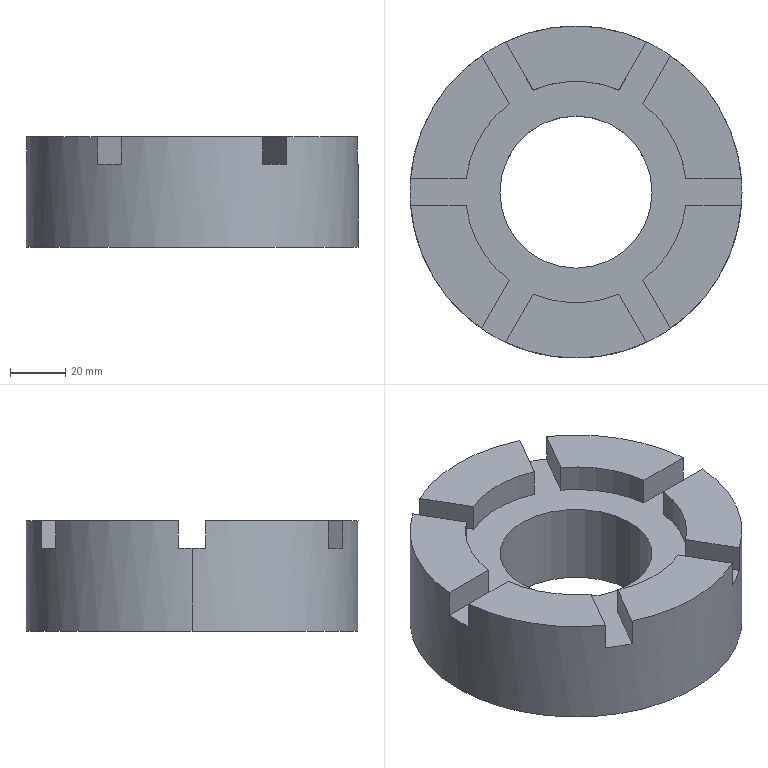Part | SolidWorks | features ICE 3, CirPattern 1, Extrusion 1 | 1 solid | 30 faces | box 120 x 120 x 40 mm | volume 318828 mm3 | plane 20 | cylinder 10 | commonest cylinder face diameters 80 x6 55 x2 120 x2
STEP:
#1=CARTESIAN_POINT('',(27.5,0.,0.));
#2=VERTEX_POINT('',#1);
#3=CARTESIAN_POINT('',(-27.5,0.,0.));
#4=VERTEX_POINT('',#3);
#5=CARTESIAN_POINT('',(0.,0.,0.));
#6=DIRECTION('',(0.,0.,-1.));
#7=DIRECTION('',(1.,0.,0.));
#8=AXIS2_PLACEMENT_3D('',#5,#6,#7);
#9=CIRCLE('',#8,27.5);
#10=EDGE_CURVE('',#2,#4,#9,.T.);
#11=ORIENTED_EDGE('',*,*,#10,.T.);
#12=CARTESIAN_POINT('',(-27.5,0.,30.));
#13=VERTEX_POINT('',#12);
#14=CARTESIAN_POINT('',(-27.5,0.,-0.001));
#15=DIRECTION('',(0.,0.,1.));
#16=VECTOR('',#15,1000.);
#17=LINE('',#14,#16);
#18=EDGE_CURVE('',#4,#13,#17,.T.);
#19=ORIENTED_EDGE('',*,*,#18,.T.);
#20=CARTESIAN_POINT('',(27.5,0.,30.));
#21=VERTEX_POINT('',#20);
#22=CARTESIAN_POINT('',(0.,0.,30.));
#23=DIRECTION('',(0.,0.,1.));
#24=DIRECTION('',(1.,0.,0.));
#25=AXIS2_PLACEMENT_3D('',#22,#23,#24);
#26=CIRCLE('',#25,27.5);
#27=EDGE_CURVE('',#13,#21,#26,.T.);
#28=ORIENTED_EDGE('',*,*,#27,.T.);
#29=CARTESIAN_POINT('',(27.5,0.,-0.001));
#30=DIRECTION('',(0.,0.,1.));
#31=VECTOR('',#30,1000.);
#32=LINE('',#29,#31);
#33=EDGE_CURVE('',#2,#21,#32,.T.);
#34=ORIENTED_EDGE('',*,*,#33,.F.);
#35=EDGE_LOOP('',(#11,#19,#28,#34));
#36=FACE_OUTER_BOUND('',#35,.T.);
#37=CARTESIAN_POINT('',(0.,0.,-0.001));
#38=DIRECTION('',(0.,0.,1.));
#39=DIRECTION('',(1.,0.,0.));
#40=AXIS2_PLACEMENT_3D('',#37,#38,#39);
#41=CYLINDRICAL_SURFACE('',#40,27.5);
#42=ADVANCED_FACE('',(#36),#41,.F.);
#43=CARTESIAN_POINT('',(60.,0.,30.));
#44=VERTEX_POINT('',#43);
#45=CARTESIAN_POINT('',(59.791,5.,30.));
#46=VERTEX_POINT('',#45);
#47=CARTESIAN_POINT('',(0.,0.,30.));
#48=DIRECTION('',(0.,0.,1.));
#49=DIRECTION('',(-1.,0.,0.));
#50=AXIS2_PLACEMENT_3D('',#47,#48,#49);
#51=CIRCLE('',#50,60.);
#52=EDGE_CURVE('',#44,#46,#51,.T.);
#53=ORIENTED_EDGE('',*,*,#52,.F.);
#54=CARTESIAN_POINT('',(60.,0.,0.));
#55=VERTEX_POINT('',#54);
#56=CARTESIAN_POINT('',(60.,0.,40.));
#57=DIRECTION('',(0.,0.,-1.));
#58=VECTOR('',#57,1000.);
#59=LINE('',#56,#58);
#60=EDGE_CURVE('',#44,#55,#59,.T.);
#61=ORIENTED_EDGE('',*,*,#60,.T.);
#62=CARTESIAN_POINT('',(-60.,0.,0.));
#63=VERTEX_POINT('',#62);
#64=CARTESIAN_POINT('',(0.,0.,0.));
#65=DIRECTION('',(0.,0.,1.));
#66=DIRECTION('',(1.,0.,0.));
#67=AXIS2_PLACEMENT_3D('',#64,#65,#66);
#68=CIRCLE('',#67,60.);
#69=EDGE_CURVE('',#55,#63,#68,.T.);
#70=ORIENTED_EDGE('',*,*,#69,.T.);
#71=CARTESIAN_POINT('',(-60.,0.,30.));
#72=VERTEX_POINT('',#71);
#73=CARTESIAN_POINT('',(-60.,0.,40.));
#74=DIRECTION('',(0.,0.,-1.));
#75=VECTOR('',#74,1000.);
#76=LINE('',#73,#75);
#77=EDGE_CURVE('',#72,#63,#76,.T.);
#78=ORIENTED_EDGE('',*,*,#77,.F.);
#79=CARTESIAN_POINT('',(-59.791,5.,30.));
#80=VERTEX_POINT('',#79);
#81=CARTESIAN_POINT('',(0.,0.,30.));
#82=DIRECTION('',(0.,0.,1.));
#83=DIRECTION('',(-1.,0.,0.));
#84=AXIS2_PLACEMENT_3D('',#81,#82,#83);
#85=CIRCLE('',#84,60.);
#86=EDGE_CURVE('',#80,#72,#85,.T.);
#87=ORIENTED_EDGE('',*,*,#86,.F.);
#88=CARTESIAN_POINT('',(-59.791,5.,40.));
#89=VERTEX_POINT('',#88);
#90=CARTESIAN_POINT('',(-59.791,5.,40.));
#91=DIRECTION('',(0.,0.,1.));
#92=VECTOR('',#91,1000.);
#93=LINE('',#90,#92);
#94=EDGE_CURVE('',#80,#89,#93,.T.);
#95=ORIENTED_EDGE('',*,*,#94,.T.);
#96=CARTESIAN_POINT('',(-34.226,49.281,40.));
#97=VERTEX_POINT('',#96);
#98=CARTESIAN_POINT('',(0.,0.,40.));
#99=DIRECTION('',(0.,0.,1.));
#100=DIRECTION('',(1.,0.,0.));
#101=AXIS2_PLACEMENT_3D('',#98,#99,#100);
#102=CIRCLE('',#101,60.);
#103=EDGE_CURVE('',#97,#89,#102,.T.);
#104=ORIENTED_EDGE('',*,*,#103,.F.);
#105=CARTESIAN_POINT('',(-34.226,49.281,30.));
#106=VERTEX_POINT('',#105);
#107=CARTESIAN_POINT('',(-34.226,49.281,40.));
#108=DIRECTION('',(0.,0.,-1.));
#109=VECTOR('',#108,1000.);
#110=LINE('',#107,#109);
#111=EDGE_CURVE('',#97,#106,#110,.T.);
#112=ORIENTED_EDGE('',*,*,#111,.T.);
#113=CARTESIAN_POINT('',(-25.566,54.281,30.));
#114=VERTEX_POINT('',#113);
#115=CARTESIAN_POINT('',(0.,0.,30.));
#116=DIRECTION('',(0.,0.,1.));
#117=DIRECTION('',(-1.,0.,0.));
#118=AXIS2_PLACEMENT_3D('',#115,#116,#117);
#119=CIRCLE('',#118,60.);
#120=EDGE_CURVE('',#114,#106,#119,.T.);
#121=ORIENTED_EDGE('',*,*,#120,.F.);
#122=CARTESIAN_POINT('',(-25.566,54.281,40.));
#123=VERTEX_POINT('',#122);
#124=CARTESIAN_POINT('',(-25.566,54.281,40.));
#125=DIRECTION('',(0.,0.,1.));
#126=VECTOR('',#125,1000.);
#127=LINE('',#124,#126);
#128=EDGE_CURVE('',#114,#123,#127,.T.);
#129=ORIENTED_EDGE('',*,*,#128,.T.);
#130=CARTESIAN_POINT('',(25.566,54.281,40.));
#131=VERTEX_POINT('',#130);
#132=CARTESIAN_POINT('',(0.,0.,40.));
#133=DIRECTION('',(0.,0.,1.));
#134=DIRECTION('',(1.,0.,0.));
#135=AXIS2_PLACEMENT_3D('',#132,#133,#134);
#136=CIRCLE('',#135,60.);
#137=EDGE_CURVE('',#131,#123,#136,.T.);
#138=ORIENTED_EDGE('',*,*,#137,.F.);
#139=CARTESIAN_POINT('',(25.566,54.281,30.));
#140=VERTEX_POINT('',#139);
#141=CARTESIAN_POINT('',(25.566,54.281,40.));
#142=DIRECTION('',(0.,0.,-1.));
#143=VECTOR('',#142,1000.);
#144=LINE('',#141,#143);
#145=EDGE_CURVE('',#131,#140,#144,.T.);
#146=ORIENTED_EDGE('',*,*,#145,.T.);
#147=CARTESIAN_POINT('',(34.226,49.281,30.));
#148=VERTEX_POINT('',#147);
#149=CARTESIAN_POINT('',(0.,0.,30.));
#150=DIRECTION('',(0.,0.,1.));
#151=DIRECTION('',(-1.,0.,0.));
#152=AXIS2_PLACEMENT_3D('',#149,#150,#151);
#153=CIRCLE('',#152,60.);
#154=EDGE_CURVE('',#148,#140,#153,.T.);
#155=ORIENTED_EDGE('',*,*,#154,.F.);
#156=CARTESIAN_POINT('',(34.226,49.281,40.));
#157=VERTEX_POINT('',#156);
#158=CARTESIAN_POINT('',(34.226,49.281,40.));
#159=DIRECTION('',(0.,0.,1.));
#160=VECTOR('',#159,1000.);
#161=LINE('',#158,#160);
#162=EDGE_CURVE('',#148,#157,#161,.T.);
#163=ORIENTED_EDGE('',*,*,#162,.T.);
#164=CARTESIAN_POINT('',(59.791,5.,40.));
#165=VERTEX_POINT('',#164);
#166=CARTESIAN_POINT('',(0.,0.,40.));
#167=DIRECTION('',(0.,0.,1.));
#168=DIRECTION('',(1.,0.,0.));
#169=AXIS2_PLACEMENT_3D('',#166,#167,#168);
#170=CIRCLE('',#169,60.);
#171=EDGE_CURVE('',#165,#157,#170,.T.);
#172=ORIENTED_EDGE('',*,*,#171,.F.);
#173=CARTESIAN_POINT('',(59.791,5.,40.));
#174=DIRECTION('',(0.,0.,-1.));
#175=VECTOR('',#174,1000.);
#176=LINE('',#173,#175);
#177=EDGE_CURVE('',#165,#46,#176,.T.);
#178=ORIENTED_EDGE('',*,*,#177,.T.);
#179=EDGE_LOOP('',(#53,#61,#70,#78,#87,#95,#104,#112,#121,#129,#138,#146,#155,#163,#172,#178));
#180=FACE_OUTER_BOUND('',#179,.T.);
#181=CARTESIAN_POINT('',(0.,0.,40.));
#182=DIRECTION('',(0.,0.,-1.));
#183=DIRECTION('',(-1.,0.,0.));
#184=AXIS2_PLACEMENT_3D('',#181,#182,#183);
#185=CYLINDRICAL_SURFACE('',#184,60.);
#186=ADVANCED_FACE('',(#180),#185,.T.);
#187=ORIENTED_EDGE('',*,*,#60,.F.);
#188=CARTESIAN_POINT('',(59.791,-5.,30.));
#189=VERTEX_POINT('',#188);
#190=CARTESIAN_POINT('',(0.,0.,30.));
#191=DIRECTION('',(0.,0.,1.));
#192=DIRECTION('',(-1.,0.,0.));
#193=AXIS2_PLACEMENT_3D('',#190,#191,#192);
#194=CIRCLE('',#193,60.);
#195=EDGE_CURVE('',#189,#44,#194,.T.);
#196=ORIENTED_EDGE('',*,*,#195,.F.);
#197=CARTESIAN_POINT('',(59.791,-5.,40.));
#198=VERTEX_POINT('',#197);
#199=CARTESIAN_POINT('',(59.791,-5.,40.));
#200=DIRECTION('',(0.,0.,1.));
#201=VECTOR('',#200,1000.);
#202=LINE('',#199,#201);
#203=EDGE_CURVE('',#189,#198,#202,.T.);
#204=ORIENTED_EDGE('',*,*,#203,.T.);
#205=CARTESIAN_POINT('',(34.226,-49.281,40.));
#206=VERTEX_POINT('',#205);
#207=CARTESIAN_POINT('',(0.,0.,40.));
#208=DIRECTION('',(0.,0.,1.));
#209=DIRECTION('',(1.,0.,0.));
#210=AXIS2_PLACEMENT_3D('',#207,#208,#209);
#211=CIRCLE('',#210,60.);
#212=EDGE_CURVE('',#206,#198,#211,.T.);
#213=ORIENTED_EDGE('',*,*,#212,.F.);
#214=CARTESIAN_POINT('',(34.226,-49.281,30.));
#215=VERTEX_POINT('',#214);
#216=CARTESIAN_POINT('',(34.226,-49.281,40.));
#217=DIRECTION('',(0.,0.,-1.));
#218=VECTOR('',#217,1000.);
#219=LINE('',#216,#218);
#220=EDGE_CURVE('',#206,#215,#219,.T.);
#221=ORIENTED_EDGE('',*,*,#220,.T.);
#222=CARTESIAN_POINT('',(25.566,-54.281,30.));
#223=VERTEX_POINT('',#222);
#224=CARTESIAN_POINT('',(0.,0.,30.));
#225=DIRECTION('',(0.,0.,1.));
#226=DIRECTION('',(-1.,0.,0.));
#227=AXIS2_PLACEMENT_3D('',#224,#225,#226);
#228=CIRCLE('',#227,60.);
#229=EDGE_CURVE('',#223,#215,#228,.T.);
#230=ORIENTED_EDGE('',*,*,#229,.F.);
#231=CARTESIAN_POINT('',(25.566,-54.281,40.));
#232=VERTEX_POINT('',#231);
#233=CARTESIAN_POINT('',(25.566,-54.281,40.));
#234=DIRECTION('',(0.,0.,1.));
#235=VECTOR('',#234,1000.);
#236=LINE('',#233,#235);
#237=EDGE_CURVE('',#223,#232,#236,.T.);
#238=ORIENTED_EDGE('',*,*,#237,.T.);
#239=CARTESIAN_POINT('',(-25.566,-54.281,40.));
#240=VERTEX_POINT('',#239);
#241=CARTESIAN_POINT('',(0.,0.,40.));
#242=DIRECTION('',(0.,0.,1.));
#243=DIRECTION('',(1.,0.,0.));
#244=AXIS2_PLACEMENT_3D('',#241,#242,#243);
#245=CIRCLE('',#244,60.);
#246=EDGE_CURVE('',#240,#232,#245,.T.);
#247=ORIENTED_EDGE('',*,*,#246,.F.);
#248=CARTESIAN_POINT('',(-25.566,-54.281,30.));
#249=VERTEX_POINT('',#248);
#250=CARTESIAN_POINT('',(-25.566,-54.281,40.));
#251=DIRECTION('',(0.,0.,-1.));
#252=VECTOR('',#251,1000.);
#253=LINE('',#250,#252);
#254=EDGE_CURVE('',#240,#249,#253,.T.);
#255=ORIENTED_EDGE('',*,*,#254,.T.);
#256=CARTESIAN_POINT('',(-34.226,-49.281,30.));
#257=VERTEX_POINT('',#256);
#258=CARTESIAN_POINT('',(0.,0.,30.));
#259=DIRECTION('',(0.,0.,1.));
#260=DIRECTION('',(-1.,0.,0.));
#261=AXIS2_PLACEMENT_3D('',#258,#259,#260);
#262=CIRCLE('',#261,60.);
#263=EDGE_CURVE('',#257,#249,#262,.T.);
#264=ORIENTED_EDGE('',*,*,#263,.F.);
#265=CARTESIAN_POINT('',(-34.226,-49.281,40.));
#266=VERTEX_POINT('',#265);
#267=CARTESIAN_POINT('',(-34.226,-49.281,40.));
#268=DIRECTION('',(0.,0.,1.));
#269=VECTOR('',#268,1000.);
#270=LINE('',#267,#269);
#271=EDGE_CURVE('',#257,#266,#270,.T.);
#272=ORIENTED_EDGE('',*,*,#271,.T.);
#273=CARTESIAN_POINT('',(-59.791,-5.,40.));
#274=VERTEX_POINT('',#273);
#275=CARTESIAN_POINT('',(0.,0.,40.));
#276=DIRECTION('',(0.,0.,1.));
#277=DIRECTION('',(1.,0.,0.));
#278=AXIS2_PLACEMENT_3D('',#275,#276,#277);
#279=CIRCLE('',#278,60.);
#280=EDGE_CURVE('',#274,#266,#279,.T.);
#281=ORIENTED_EDGE('',*,*,#280,.F.);
#282=CARTESIAN_POINT('',(-59.791,-5.,30.));
#283=VERTEX_POINT('',#282);
#284=CARTESIAN_POINT('',(-59.791,-5.,40.));
#285=DIRECTION('',(0.,0.,-1.));
#286=VECTOR('',#285,1000.);
#287=LINE('',#284,#286);
#288=EDGE_CURVE('',#274,#283,#287,.T.);
#289=ORIENTED_EDGE('',*,*,#288,.T.);
#290=CARTESIAN_POINT('',(0.,0.,30.));
#291=DIRECTION('',(0.,0.,1.));
#292=DIRECTION('',(-1.,0.,0.));
#293=AXIS2_PLACEMENT_3D('',#290,#291,#292);
#294=CIRCLE('',#293,60.);
#295=EDGE_CURVE('',#72,#283,#294,.T.);
#296=ORIENTED_EDGE('',*,*,#295,.F.);
#297=ORIENTED_EDGE('',*,*,#77,.T.);
#298=CARTESIAN_POINT('',(0.,0.,0.));
#299=DIRECTION('',(0.,0.,1.));
#300=DIRECTION('',(1.,0.,0.));
#301=AXIS2_PLACEMENT_3D('',#298,#299,#300);
#302=CIRCLE('',#301,60.);
#303=EDGE_CURVE('',#63,#55,#302,.T.);
#304=ORIENTED_EDGE('',*,*,#303,.T.);
#305=EDGE_LOOP('',(#187,#196,#204,#213,#221,#230,#238,#247,#255,#264,#272,#281,#289,#296,#297,#304));
#306=FACE_OUTER_BOUND('',#305,.T.);
#307=CARTESIAN_POINT('',(0.,0.,40.));
#308=DIRECTION('',(0.,0.,-1.));
#309=DIRECTION('',(-1.,0.,0.));
#310=AXIS2_PLACEMENT_3D('',#307,#308,#309);
#311=CYLINDRICAL_SURFACE('',#310,60.);
#312=ADVANCED_FACE('',(#306),#311,.T.);
#313=ORIENTED_EDGE('',*,*,#246,.T.);
#314=CARTESIAN_POINT('',(15.513,-36.869,40.));
#315=VERTEX_POINT('',#314);
#316=CARTESIAN_POINT('',(33.17,-67.452,40.));
#317=DIRECTION('',(0.5,-0.866,0.));
#318=VECTOR('',#317,1000.);
#319=LINE('',#316,#318);
#320=EDGE_CURVE('',#315,#232,#319,.T.);
#321=ORIENTED_EDGE('',*,*,#320,.F.);
#322=CARTESIAN_POINT('',(-15.513,-36.869,40.));
#323=VERTEX_POINT('',#322);
#324=CARTESIAN_POINT('',(0.,0.,40.));
#325=DIRECTION('',(0.,0.,1.));
#326=DIRECTION('',(1.,0.,0.));
#327=AXIS2_PLACEMENT_3D('',#324,#325,#326);
#328=CIRCLE('',#327,40.);
#329=EDGE_CURVE('',#323,#315,#328,.T.);
#330=ORIENTED_EDGE('',*,*,#329,.F.);
#331=CARTESIAN_POINT('',(41.83,62.452,40.));
#332=DIRECTION('',(0.5,0.866,0.));
#333=VECTOR('',#332,1000.);
#334=LINE('',#331,#333);
#335=EDGE_CURVE('',#240,#323,#334,.T.);
#336=ORIENTED_EDGE('',*,*,#335,.F.);
#337=EDGE_LOOP('',(#313,#321,#330,#336));
#338=FACE_OUTER_BOUND('',#337,.T.);
#339=CARTESIAN_POINT('',(0.,0.,40.));
#340=DIRECTION('',(0.,0.,1.));
#341=DIRECTION('',(1.,0.,0.));
#342=AXIS2_PLACEMENT_3D('',#339,#340,#341);
#343=PLANE('',#342);
#344=ADVANCED_FACE('',(#338),#343,.T.);
#345=CARTESIAN_POINT('',(24.173,-31.869,40.));
#346=VERTEX_POINT('',#345);
#347=CARTESIAN_POINT('',(39.686,-5.,40.));
#348=VERTEX_POINT('',#347);
#349=CARTESIAN_POINT('',(0.,0.,40.));
#350=DIRECTION('',(0.,0.,1.));
#351=DIRECTION('',(1.,0.,0.));
#352=AXIS2_PLACEMENT_3D('',#349,#350,#351);
#353=CIRCLE('',#352,40.);
#354=EDGE_CURVE('',#346,#348,#353,.T.);
#355=ORIENTED_EDGE('',*,*,#354,.F.);
#356=CARTESIAN_POINT('',(41.83,-62.452,40.));
#357=DIRECTION('',(-0.5,0.866,0.));
#358=VECTOR('',#357,1000.);
#359=LINE('',#356,#358);
#360=EDGE_CURVE('',#206,#346,#359,.T.);
#361=ORIENTED_EDGE('',*,*,#360,.F.);
#362=ORIENTED_EDGE('',*,*,#212,.T.);
#363=CARTESIAN_POINT('',(-75.,-5.,40.));
#364=DIRECTION('',(1.,0.,0.));
#365=VECTOR('',#364,1000.);
#366=LINE('',#363,#365);
#367=EDGE_CURVE('',#348,#198,#366,.T.);
#368=ORIENTED_EDGE('',*,*,#367,.F.);
#369=EDGE_LOOP('',(#355,#361,#362,#368));
#370=FACE_OUTER_BOUND('',#369,.T.);
#371=CARTESIAN_POINT('',(0.,0.,40.));
#372=DIRECTION('',(0.,0.,1.));
#373=DIRECTION('',(1.,0.,0.));
#374=AXIS2_PLACEMENT_3D('',#371,#372,#373);
#375=PLANE('',#374);
#376=ADVANCED_FACE('',(#370),#375,.T.);
#377=ORIENTED_EDGE('',*,*,#280,.T.);
#378=CARTESIAN_POINT('',(-24.173,-31.869,40.));
#379=VERTEX_POINT('',#378);
#380=CARTESIAN_POINT('',(33.17,67.452,40.));
#381=DIRECTION('',(-0.5,-0.866,0.));
#382=VECTOR('',#381,1000.);
#383=LINE('',#380,#382);
#384=EDGE_CURVE('',#379,#266,#383,.T.);
#385=ORIENTED_EDGE('',*,*,#384,.F.);
#386=CARTESIAN_POINT('',(-39.686,-5.,40.));
#387=VERTEX_POINT('',#386);
#388=CARTESIAN_POINT('',(0.,0.,40.));
#389=DIRECTION('',(0.,0.,1.));
#390=DIRECTION('',(1.,0.,0.));
#391=AXIS2_PLACEMENT_3D('',#388,#389,#390);
#392=CIRCLE('',#391,40.);
#393=EDGE_CURVE('',#387,#379,#392,.T.);
#394=ORIENTED_EDGE('',*,*,#393,.F.);
#395=CARTESIAN_POINT('',(-75.,-5.,40.));
#396=DIRECTION('',(1.,0.,0.));
#397=VECTOR('',#396,1000.);
#398=LINE('',#395,#397);
#399=EDGE_CURVE('',#274,#387,#398,.T.);
#400=ORIENTED_EDGE('',*,*,#399,.F.);
#401=EDGE_LOOP('',(#377,#385,#394,#400));
#402=FACE_OUTER_BOUND('',#401,.T.);
#403=CARTESIAN_POINT('',(0.,0.,40.));
#404=DIRECTION('',(0.,0.,1.));
#405=DIRECTION('',(1.,0.,0.));
#406=AXIS2_PLACEMENT_3D('',#403,#404,#405);
#407=PLANE('',#406);
#408=ADVANCED_FACE('',(#402),#407,.T.);
#409=ORIENTED_EDGE('',*,*,#137,.T.);
#410=CARTESIAN_POINT('',(-15.513,36.869,40.));
#411=VERTEX_POINT('',#410);
#412=CARTESIAN_POINT('',(41.83,-62.452,40.));
#413=DIRECTION('',(-0.5,0.866,0.));
#414=VECTOR('',#413,1000.);
#415=LINE('',#412,#414);
#416=EDGE_CURVE('',#411,#123,#415,.T.);
#417=ORIENTED_EDGE('',*,*,#416,.F.);
#418=CARTESIAN_POINT('',(15.513,36.869,40.));
#419=VERTEX_POINT('',#418);
#420=CARTESIAN_POINT('',(0.,0.,40.));
#421=DIRECTION('',(0.,0.,1.));
#422=DIRECTION('',(1.,0.,0.));
#423=AXIS2_PLACEMENT_3D('',#420,#421,#422);
#424=CIRCLE('',#423,40.);
#425=EDGE_CURVE('',#419,#411,#424,.T.);
#426=ORIENTED_EDGE('',*,*,#425,.F.);
#427=CARTESIAN_POINT('',(33.17,67.452,40.));
#428=DIRECTION('',(-0.5,-0.866,0.));
#429=VECTOR('',#428,1000.);
#430=LINE('',#427,#429);
#431=EDGE_CURVE('',#131,#419,#430,.T.);
#432=ORIENTED_EDGE('',*,*,#431,.F.);
#433=EDGE_LOOP('',(#409,#417,#426,#432));
#434=FACE_OUTER_BOUND('',#433,.T.);
#435=CARTESIAN_POINT('',(0.,0.,40.));
#436=DIRECTION('',(0.,0.,1.));
#437=DIRECTION('',(1.,0.,0.));
#438=AXIS2_PLACEMENT_3D('',#435,#436,#437);
#439=PLANE('',#438);
#440=ADVANCED_FACE('',(#434),#439,.T.);
#441=CARTESIAN_POINT('',(-24.173,31.869,40.));
#442=VERTEX_POINT('',#441);
#443=CARTESIAN_POINT('',(-39.686,5.,40.));
#444=VERTEX_POINT('',#443);
#445=CARTESIAN_POINT('',(0.,0.,40.));
#446=DIRECTION('',(0.,0.,1.));
#447=DIRECTION('',(1.,0.,0.));
#448=AXIS2_PLACEMENT_3D('',#445,#446,#447);
#449=CIRCLE('',#448,40.);
#450=EDGE_CURVE('',#442,#444,#449,.T.);
#451=ORIENTED_EDGE('',*,*,#450,.F.);
#452=CARTESIAN_POINT('',(33.17,-67.452,40.));
#453=DIRECTION('',(0.5,-0.866,0.));
#454=VECTOR('',#453,1000.);
#455=LINE('',#452,#454);
#456=EDGE_CURVE('',#97,#442,#455,.T.);
#457=ORIENTED_EDGE('',*,*,#456,.F.);
#458=ORIENTED_EDGE('',*,*,#103,.T.);
#459=CARTESIAN_POINT('',(-75.,5.,40.));
#460=DIRECTION('',(-1.,0.,0.));
#461=VECTOR('',#460,1000.);
#462=LINE('',#459,#461);
#463=EDGE_CURVE('',#444,#89,#462,.T.);
#464=ORIENTED_EDGE('',*,*,#463,.F.);
#465=EDGE_LOOP('',(#451,#457,#458,#464));
#466=FACE_OUTER_BOUND('',#465,.T.);
#467=CARTESIAN_POINT('',(0.,0.,40.));
#468=DIRECTION('',(0.,0.,1.));
#469=DIRECTION('',(1.,0.,0.));
#470=AXIS2_PLACEMENT_3D('',#467,#468,#469);
#471=PLANE('',#470);
#472=ADVANCED_FACE('',(#466),#471,.T.);
#473=ORIENTED_EDGE('',*,*,#171,.T.);
#474=CARTESIAN_POINT('',(24.173,31.869,40.));
#475=VERTEX_POINT('',#474);
#476=CARTESIAN_POINT('',(41.83,62.452,40.));
#477=DIRECTION('',(0.5,0.866,0.));
#478=VECTOR('',#477,1000.);
#479=LINE('',#476,#478);
#480=EDGE_CURVE('',#475,#157,#479,.T.);
#481=ORIENTED_EDGE('',*,*,#480,.F.);
#482=CARTESIAN_POINT('',(39.686,5.,40.));
#483=VERTEX_POINT('',#482);
#484=CARTESIAN_POINT('',(0.,0.,40.));
#485=DIRECTION('',(0.,0.,1.));
#486=DIRECTION('',(1.,0.,0.));
#487=AXIS2_PLACEMENT_3D('',#484,#485,#486);
#488=CIRCLE('',#487,40.);
#489=EDGE_CURVE('',#483,#475,#488,.T.);
#490=ORIENTED_EDGE('',*,*,#489,.F.);
#491=CARTESIAN_POINT('',(-75.,5.,40.));
#492=DIRECTION('',(-1.,0.,0.));
#493=VECTOR('',#492,1000.);
#494=LINE('',#491,#493);
#495=EDGE_CURVE('',#165,#483,#494,.T.);
#496=ORIENTED_EDGE('',*,*,#495,.F.);
#497=EDGE_LOOP('',(#473,#481,#490,#496));
#498=FACE_OUTER_BOUND('',#497,.T.);
#499=CARTESIAN_POINT('',(0.,0.,40.));
#500=DIRECTION('',(0.,0.,1.));
#501=DIRECTION('',(1.,0.,0.));
#502=AXIS2_PLACEMENT_3D('',#499,#500,#501);
#503=PLANE('',#502);
#504=ADVANCED_FACE('',(#498),#503,.T.);
#505=CARTESIAN_POINT('',(15.513,-36.869,30.));
#506=VERTEX_POINT('',#505);
#507=CARTESIAN_POINT('',(15.513,-36.869,30.));
#508=DIRECTION('',(0.,0.,-1.));
#509=VECTOR('',#508,1000.);
#510=LINE('',#507,#509);
#511=EDGE_CURVE('',#315,#506,#510,.T.);
#512=ORIENTED_EDGE('',*,*,#511,.T.);
#513=CARTESIAN_POINT('',(-15.513,-36.869,30.));
#514=VERTEX_POINT('',#513);
#515=CARTESIAN_POINT('',(0.,0.,30.));
#516=DIRECTION('',(0.,0.,1.));
#517=DIRECTION('',(1.,0.,0.));
#518=AXIS2_PLACEMENT_3D('',#515,#516,#517);
#519=CIRCLE('',#518,40.);
#520=EDGE_CURVE('',#514,#506,#519,.T.);
#521=ORIENTED_EDGE('',*,*,#520,.F.);
#522=CARTESIAN_POINT('',(-15.513,-36.869,30.));
#523=DIRECTION('',(0.,0.,1.));
#524=VECTOR('',#523,1000.);
#525=LINE('',#522,#524);
#526=EDGE_CURVE('',#514,#323,#525,.T.);
#527=ORIENTED_EDGE('',*,*,#526,.T.);
#528=ORIENTED_EDGE('',*,*,#329,.T.);
#529=EDGE_LOOP('',(#512,#521,#527,#528));
#530=FACE_OUTER_BOUND('',#529,.T.);
#531=CARTESIAN_POINT('',(0.,0.,30.));
#532=DIRECTION('',(0.,0.,1.));
#533=DIRECTION('',(1.,0.,0.));
#534=AXIS2_PLACEMENT_3D('',#531,#532,#533);
#535=CYLINDRICAL_SURFACE('',#534,40.);
#536=ADVANCED_FACE('',(#530),#535,.F.);
#537=CARTESIAN_POINT('',(24.173,-31.869,30.));
#538=VERTEX_POINT('',#537);
#539=CARTESIAN_POINT('',(24.173,-31.869,30.));
#540=DIRECTION('',(0.,0.,1.));
#541=VECTOR('',#540,1000.);
#542=LINE('',#539,#541);
#543=EDGE_CURVE('',#538,#346,#542,.T.);
#544=ORIENTED_EDGE('',*,*,#543,.T.);
#545=ORIENTED_EDGE('',*,*,#354,.T.);
#546=CARTESIAN_POINT('',(39.686,-5.,30.));
#547=VERTEX_POINT('',#546);
#548=CARTESIAN_POINT('',(39.686,-5.,30.));
#549=DIRECTION('',(0.,0.,-1.));
#550=VECTOR('',#549,1000.);
#551=LINE('',#548,#550);
#552=EDGE_CURVE('',#348,#547,#551,.T.);
#553=ORIENTED_EDGE('',*,*,#552,.T.);
#554=CARTESIAN_POINT('',(0.,0.,30.));
#555=DIRECTION('',(0.,0.,1.));
#556=DIRECTION('',(1.,0.,0.));
#557=AXIS2_PLACEMENT_3D('',#554,#555,#556);
#558=CIRCLE('',#557,40.);
#559=EDGE_CURVE('',#538,#547,#558,.T.);
#560=ORIENTED_EDGE('',*,*,#559,.F.);
#561=EDGE_LOOP('',(#544,#545,#553,#560));
#562=FACE_OUTER_BOUND('',#561,.T.);
#563=CARTESIAN_POINT('',(0.,0.,30.));
#564=DIRECTION('',(0.,0.,1.));
#565=DIRECTION('',(1.,0.,0.));
#566=AXIS2_PLACEMENT_3D('',#563,#564,#565);
#567=CYLINDRICAL_SURFACE('',#566,40.);
#568=ADVANCED_FACE('',(#562),#567,.F.);
#569=CARTESIAN_POINT('',(-24.173,-31.869,30.));
#570=VERTEX_POINT('',#569);
#571=CARTESIAN_POINT('',(-24.173,-31.869,30.));
#572=DIRECTION('',(0.,0.,-1.));
#573=VECTOR('',#572,1000.);
#574=LINE('',#571,#573);
#575=EDGE_CURVE('',#379,#570,#574,.T.);
#576=ORIENTED_EDGE('',*,*,#575,.T.);
#577=CARTESIAN_POINT('',(-39.686,-5.,30.));
#578=VERTEX_POINT('',#577);
#579=CARTESIAN_POINT('',(0.,0.,30.));
#580=DIRECTION('',(0.,0.,1.));
#581=DIRECTION('',(1.,0.,0.));
#582=AXIS2_PLACEMENT_3D('',#579,#580,#581);
#583=CIRCLE('',#582,40.);
#584=EDGE_CURVE('',#578,#570,#583,.T.);
#585=ORIENTED_EDGE('',*,*,#584,.F.);
#586=CARTESIAN_POINT('',(-39.686,-5.,30.));
#587=DIRECTION('',(0.,0.,1.));
#588=VECTOR('',#587,1000.);
#589=LINE('',#586,#588);
#590=EDGE_CURVE('',#578,#387,#589,.T.);
#591=ORIENTED_EDGE('',*,*,#590,.T.);
#592=ORIENTED_EDGE('',*,*,#393,.T.);
#593=EDGE_LOOP('',(#576,#585,#591,#592));
#594=FACE_OUTER_BOUND('',#593,.T.);
#595=CARTESIAN_POINT('',(0.,0.,30.));
#596=DIRECTION('',(0.,0.,1.));
#597=DIRECTION('',(1.,0.,0.));
#598=AXIS2_PLACEMENT_3D('',#595,#596,#597);
#599=CYLINDRICAL_SURFACE('',#598,40.);
#600=ADVANCED_FACE('',(#594),#599,.F.);
#601=CARTESIAN_POINT('',(-15.513,36.869,30.));
#602=VERTEX_POINT('',#601);
#603=CARTESIAN_POINT('',(-15.513,36.869,30.));
#604=DIRECTION('',(0.,0.,-1.));
#605=VECTOR('',#604,1000.);
#606=LINE('',#603,#605);
#607=EDGE_CURVE('',#411,#602,#606,.T.);
#608=ORIENTED_EDGE('',*,*,#607,.T.);
#609=CARTESIAN_POINT('',(15.513,36.869,30.));
#610=VERTEX_POINT('',#609);
#611=CARTESIAN_POINT('',(0.,0.,30.));
#612=DIRECTION('',(0.,0.,1.));
#613=DIRECTION('',(1.,0.,0.));
#614=AXIS2_PLACEMENT_3D('',#611,#612,#613);
#615=CIRCLE('',#614,40.);
#616=EDGE_CURVE('',#610,#602,#615,.T.);
#617=ORIENTED_EDGE('',*,*,#616,.F.);
#618=CARTESIAN_POINT('',(15.513,36.869,30.));
#619=DIRECTION('',(0.,0.,1.));
#620=VECTOR('',#619,1000.);
#621=LINE('',#618,#620);
#622=EDGE_CURVE('',#610,#419,#621,.T.);
#623=ORIENTED_EDGE('',*,*,#622,.T.);
#624=ORIENTED_EDGE('',*,*,#425,.T.);
#625=EDGE_LOOP('',(#608,#617,#623,#624));
#626=FACE_OUTER_BOUND('',#625,.T.);
#627=CARTESIAN_POINT('',(0.,0.,30.));
#628=DIRECTION('',(0.,0.,1.));
#629=DIRECTION('',(1.,0.,0.));
#630=AXIS2_PLACEMENT_3D('',#627,#628,#629);
#631=CYLINDRICAL_SURFACE('',#630,40.);
#632=ADVANCED_FACE('',(#626),#631,.F.);
#633=CARTESIAN_POINT('',(-24.173,31.869,30.));
#634=VERTEX_POINT('',#633);
#635=CARTESIAN_POINT('',(-24.173,31.869,30.));
#636=DIRECTION('',(0.,0.,1.));
#637=VECTOR('',#636,1000.);
#638=LINE('',#635,#637);
#639=EDGE_CURVE('',#634,#442,#638,.T.);
#640=ORIENTED_EDGE('',*,*,#639,.T.);
#641=ORIENTED_EDGE('',*,*,#450,.T.);
#642=CARTESIAN_POINT('',(-39.686,5.,30.));
#643=VERTEX_POINT('',#642);
#644=CARTESIAN_POINT('',(-39.686,5.,30.));
#645=DIRECTION('',(0.,0.,-1.));
#646=VECTOR('',#645,1000.);
#647=LINE('',#644,#646);
#648=EDGE_CURVE('',#444,#643,#647,.T.);
#649=ORIENTED_EDGE('',*,*,#648,.T.);
#650=CARTESIAN_POINT('',(0.,0.,30.));
#651=DIRECTION('',(0.,0.,1.));
#652=DIRECTION('',(1.,0.,0.));
#653=AXIS2_PLACEMENT_3D('',#650,#651,#652);
#654=CIRCLE('',#653,40.);
#655=EDGE_CURVE('',#634,#643,#654,.T.);
#656=ORIENTED_EDGE('',*,*,#655,.F.);
#657=EDGE_LOOP('',(#640,#641,#649,#656));
#658=FACE_OUTER_BOUND('',#657,.T.);
#659=CARTESIAN_POINT('',(0.,0.,30.));
#660=DIRECTION('',(0.,0.,1.));
#661=DIRECTION('',(1.,0.,0.));
#662=AXIS2_PLACEMENT_3D('',#659,#660,#661);
#663=CYLINDRICAL_SURFACE('',#662,40.);
#664=ADVANCED_FACE('',(#658),#663,.F.);
#665=CARTESIAN_POINT('',(24.173,31.869,30.));
#666=VERTEX_POINT('',#665);
#667=CARTESIAN_POINT('',(24.173,31.869,30.));
#668=DIRECTION('',(0.,0.,-1.));
#669=VECTOR('',#668,1000.);
#670=LINE('',#667,#669);
#671=EDGE_CURVE('',#475,#666,#670,.T.);
#672=ORIENTED_EDGE('',*,*,#671,.T.);
#673=CARTESIAN_POINT('',(39.686,5.,30.));
#674=VERTEX_POINT('',#673);
#675=CARTESIAN_POINT('',(0.,0.,30.));
#676=DIRECTION('',(0.,0.,1.));
#677=DIRECTION('',(1.,0.,0.));
#678=AXIS2_PLACEMENT_3D('',#675,#676,#677);
#679=CIRCLE('',#678,40.);
#680=EDGE_CURVE('',#674,#666,#679,.T.);
#681=ORIENTED_EDGE('',*,*,#680,.F.);
#682=CARTESIAN_POINT('',(39.686,5.,30.));
#683=DIRECTION('',(0.,0.,1.));
#684=VECTOR('',#683,1000.);
#685=LINE('',#682,#684);
#686=EDGE_CURVE('',#674,#483,#685,.T.);
#687=ORIENTED_EDGE('',*,*,#686,.T.);
#688=ORIENTED_EDGE('',*,*,#489,.T.);
#689=EDGE_LOOP('',(#672,#681,#687,#688));
#690=FACE_OUTER_BOUND('',#689,.T.);
#691=CARTESIAN_POINT('',(0.,0.,30.));
#692=DIRECTION('',(0.,0.,1.));
#693=DIRECTION('',(1.,0.,0.));
#694=AXIS2_PLACEMENT_3D('',#691,#692,#693);
#695=CYLINDRICAL_SURFACE('',#694,40.);
#696=ADVANCED_FACE('',(#690),#695,.F.);
#697=ORIENTED_EDGE('',*,*,#10,.F.);
#698=CARTESIAN_POINT('',(0.,0.,0.));
#699=DIRECTION('',(0.,0.,-1.));
#700=DIRECTION('',(1.,0.,0.));
#701=AXIS2_PLACEMENT_3D('',#698,#699,#700);
#702=CIRCLE('',#701,27.5);
#703=EDGE_CURVE('',#4,#2,#702,.T.);
#704=ORIENTED_EDGE('',*,*,#703,.F.);
#705=EDGE_LOOP('',(#697,#704));
#706=FACE_BOUND('',#705,.T.);
#707=ORIENTED_EDGE('',*,*,#303,.F.);
#708=ORIENTED_EDGE('',*,*,#69,.F.);
#709=EDGE_LOOP('',(#707,#708));
#710=FACE_OUTER_BOUND('',#709,.T.);
#711=CARTESIAN_POINT('',(0.,0.,0.));
#712=DIRECTION('',(0.,0.,1.));
#713=DIRECTION('',(1.,0.,0.));
#714=AXIS2_PLACEMENT_3D('',#711,#712,#713);
#715=PLANE('',#714);
#716=ADVANCED_FACE('',(#706,#710),#715,.F.);
#717=CARTESIAN_POINT('',(0.,0.,30.));
#718=DIRECTION('',(0.,0.,1.));
#719=DIRECTION('',(1.,0.,0.));
#720=AXIS2_PLACEMENT_3D('',#717,#718,#719);
#721=CIRCLE('',#720,27.5);
#722=EDGE_CURVE('',#21,#13,#721,.T.);
#723=ORIENTED_EDGE('',*,*,#722,.F.);
#724=ORIENTED_EDGE('',*,*,#27,.F.);
#725=EDGE_LOOP('',(#723,#724));
#726=FACE_BOUND('',#725,.T.);
#727=ORIENTED_EDGE('',*,*,#680,.T.);
#728=CARTESIAN_POINT('',(41.83,62.452,30.));
#729=DIRECTION('',(0.5,0.866,0.));
#730=VECTOR('',#729,1000.);
#731=LINE('',#728,#730);
#732=EDGE_CURVE('',#666,#148,#731,.T.);
#733=ORIENTED_EDGE('',*,*,#732,.T.);
#734=ORIENTED_EDGE('',*,*,#154,.T.);
#735=CARTESIAN_POINT('',(33.17,67.452,30.));
#736=DIRECTION('',(-0.5,-0.866,0.));
#737=VECTOR('',#736,1000.);
#738=LINE('',#735,#737);
#739=EDGE_CURVE('',#140,#610,#738,.T.);
#740=ORIENTED_EDGE('',*,*,#739,.T.);
#741=ORIENTED_EDGE('',*,*,#616,.T.);
#742=CARTESIAN_POINT('',(41.83,-62.452,30.));
#743=DIRECTION('',(-0.5,0.866,0.));
#744=VECTOR('',#743,1000.);
#745=LINE('',#742,#744);
#746=EDGE_CURVE('',#602,#114,#745,.T.);
#747=ORIENTED_EDGE('',*,*,#746,.T.);
#748=ORIENTED_EDGE('',*,*,#120,.T.);
#749=CARTESIAN_POINT('',(33.17,-67.452,30.));
#750=DIRECTION('',(0.5,-0.866,0.));
#751=VECTOR('',#750,1000.);
#752=LINE('',#749,#751);
#753=EDGE_CURVE('',#106,#634,#752,.T.);
#754=ORIENTED_EDGE('',*,*,#753,.T.);
#755=ORIENTED_EDGE('',*,*,#655,.T.);
#756=CARTESIAN_POINT('',(-75.,5.,30.));
#757=DIRECTION('',(-1.,0.,0.));
#758=VECTOR('',#757,1000.);
#759=LINE('',#756,#758);
#760=EDGE_CURVE('',#643,#80,#759,.T.);
#761=ORIENTED_EDGE('',*,*,#760,.T.);
#762=ORIENTED_EDGE('',*,*,#86,.T.);
#763=ORIENTED_EDGE('',*,*,#295,.T.);
#764=CARTESIAN_POINT('',(-75.,-5.,30.));
#765=DIRECTION('',(1.,0.,0.));
#766=VECTOR('',#765,1000.);
#767=LINE('',#764,#766);
#768=EDGE_CURVE('',#283,#578,#767,.T.);
#769=ORIENTED_EDGE('',*,*,#768,.T.);
#770=ORIENTED_EDGE('',*,*,#584,.T.);
#771=CARTESIAN_POINT('',(33.17,67.452,30.));
#772=DIRECTION('',(-0.5,-0.866,0.));
#773=VECTOR('',#772,1000.);
#774=LINE('',#771,#773);
#775=EDGE_CURVE('',#570,#257,#774,.T.);
#776=ORIENTED_EDGE('',*,*,#775,.T.);
#777=ORIENTED_EDGE('',*,*,#263,.T.);
#778=CARTESIAN_POINT('',(41.83,62.452,30.));
#779=DIRECTION('',(0.5,0.866,0.));
#780=VECTOR('',#779,1000.);
#781=LINE('',#778,#780);
#782=EDGE_CURVE('',#249,#514,#781,.T.);
#783=ORIENTED_EDGE('',*,*,#782,.T.);
#784=ORIENTED_EDGE('',*,*,#520,.T.);
#785=CARTESIAN_POINT('',(33.17,-67.452,30.));
#786=DIRECTION('',(0.5,-0.866,0.));
#787=VECTOR('',#786,1000.);
#788=LINE('',#785,#787);
#789=EDGE_CURVE('',#506,#223,#788,.T.);
#790=ORIENTED_EDGE('',*,*,#789,.T.);
#791=ORIENTED_EDGE('',*,*,#229,.T.);
#792=CARTESIAN_POINT('',(41.83,-62.452,30.));
#793=DIRECTION('',(-0.5,0.866,0.));
#794=VECTOR('',#793,1000.);
#795=LINE('',#792,#794);
#796=EDGE_CURVE('',#215,#538,#795,.T.);
#797=ORIENTED_EDGE('',*,*,#796,.T.);
#798=ORIENTED_EDGE('',*,*,#559,.T.);
#799=CARTESIAN_POINT('',(-75.,-5.,30.));
#800=DIRECTION('',(1.,0.,0.));
#801=VECTOR('',#800,1000.);
#802=LINE('',#799,#801);
#803=EDGE_CURVE('',#547,#189,#802,.T.);
#804=ORIENTED_EDGE('',*,*,#803,.T.);
#805=ORIENTED_EDGE('',*,*,#195,.T.);
#806=ORIENTED_EDGE('',*,*,#52,.T.);
#807=CARTESIAN_POINT('',(-75.,5.,30.));
#808=DIRECTION('',(-1.,0.,0.));
#809=VECTOR('',#808,1000.);
#810=LINE('',#807,#809);
#811=EDGE_CURVE('',#46,#674,#810,.T.);
#812=ORIENTED_EDGE('',*,*,#811,.T.);
#813=EDGE_LOOP('',(#727,#733,#734,#740,#741,#747,#748,#754,#755,#761,#762,#763,#769,#770,#776,#777,#783,#784,#790,#791,#797,#798,#804,#805,#806,#812));
#814=FACE_OUTER_BOUND('',#813,.T.);
#815=CARTESIAN_POINT('',(0.,0.,30.));
#816=DIRECTION('',(0.,0.,1.));
#817=DIRECTION('',(1.,0.,0.));
#818=AXIS2_PLACEMENT_3D('',#815,#816,#817);
#819=PLANE('',#818);
#820=ADVANCED_FACE('',(#726,#814),#819,.T.);
#821=ORIENTED_EDGE('',*,*,#18,.F.);
#822=ORIENTED_EDGE('',*,*,#703,.T.);
#823=ORIENTED_EDGE('',*,*,#33,.T.);
#824=ORIENTED_EDGE('',*,*,#722,.T.);
#825=EDGE_LOOP('',(#821,#822,#823,#824));
#826=FACE_OUTER_BOUND('',#825,.T.);
#827=CARTESIAN_POINT('',(0.,0.,-0.001));
#828=DIRECTION('',(0.,0.,1.));
#829=DIRECTION('',(1.,0.,0.));
#830=AXIS2_PLACEMENT_3D('',#827,#828,#829);
#831=CYLINDRICAL_SURFACE('',#830,27.5);
#832=ADVANCED_FACE('',(#826),#831,.F.);
#833=ORIENTED_EDGE('',*,*,#495,.T.);
#834=ORIENTED_EDGE('',*,*,#686,.F.);
#835=ORIENTED_EDGE('',*,*,#811,.F.);
#836=ORIENTED_EDGE('',*,*,#177,.F.);
#837=EDGE_LOOP('',(#833,#834,#835,#836));
#838=FACE_OUTER_BOUND('',#837,.T.);
#839=CARTESIAN_POINT('',(-75.,5.,40.001));
#840=DIRECTION('',(0.,-1.,0.));
#841=DIRECTION('',(0.,0.,-1.));
#842=AXIS2_PLACEMENT_3D('',#839,#840,#841);
#843=PLANE('',#842);
#844=ADVANCED_FACE('',(#838),#843,.T.);
#845=ORIENTED_EDGE('',*,*,#803,.F.);
#846=ORIENTED_EDGE('',*,*,#552,.F.);
#847=ORIENTED_EDGE('',*,*,#367,.T.);
#848=ORIENTED_EDGE('',*,*,#203,.F.);
#849=EDGE_LOOP('',(#845,#846,#847,#848));
#850=FACE_OUTER_BOUND('',#849,.T.);
#851=CARTESIAN_POINT('',(-75.,-5.,40.001));
#852=DIRECTION('',(0.,1.,0.));
#853=DIRECTION('',(0.,0.,1.));
#854=AXIS2_PLACEMENT_3D('',#851,#852,#853);
#855=PLANE('',#854);
#856=ADVANCED_FACE('',(#850),#855,.T.);
#857=ORIENTED_EDGE('',*,*,#399,.T.);
#858=ORIENTED_EDGE('',*,*,#590,.F.);
#859=ORIENTED_EDGE('',*,*,#768,.F.);
#860=ORIENTED_EDGE('',*,*,#288,.F.);
#861=EDGE_LOOP('',(#857,#858,#859,#860));
#862=FACE_OUTER_BOUND('',#861,.T.);
#863=CARTESIAN_POINT('',(-75.,-5.,40.001));
#864=DIRECTION('',(0.,1.,0.));
#865=DIRECTION('',(0.,0.,1.));
#866=AXIS2_PLACEMENT_3D('',#863,#864,#865);
#867=PLANE('',#866);
#868=ADVANCED_FACE('',(#862),#867,.T.);
#869=ORIENTED_EDGE('',*,*,#760,.F.);
#870=ORIENTED_EDGE('',*,*,#648,.F.);
#871=ORIENTED_EDGE('',*,*,#463,.T.);
#872=ORIENTED_EDGE('',*,*,#94,.F.);
#873=EDGE_LOOP('',(#869,#870,#871,#872));
#874=FACE_OUTER_BOUND('',#873,.T.);
#875=CARTESIAN_POINT('',(-75.,5.,40.001));
#876=DIRECTION('',(0.,-1.,0.));
#877=DIRECTION('',(0.,0.,-1.));
#878=AXIS2_PLACEMENT_3D('',#875,#876,#877);
#879=PLANE('',#878);
#880=ADVANCED_FACE('',(#874),#879,.T.);
#881=ORIENTED_EDGE('',*,*,#431,.T.);
#882=ORIENTED_EDGE('',*,*,#622,.F.);
#883=ORIENTED_EDGE('',*,*,#739,.F.);
#884=ORIENTED_EDGE('',*,*,#145,.F.);
#885=EDGE_LOOP('',(#881,#882,#883,#884));
#886=FACE_OUTER_BOUND('',#885,.T.);
#887=CARTESIAN_POINT('',(33.17,67.452,40.001));
#888=DIRECTION('',(0.866,-0.5,0.));
#889=DIRECTION('',(0.5,0.866,0.));
#890=AXIS2_PLACEMENT_3D('',#887,#888,#889);
#891=PLANE('',#890);
#892=ADVANCED_FACE('',(#886),#891,.T.);
#893=ORIENTED_EDGE('',*,*,#732,.F.);
#894=ORIENTED_EDGE('',*,*,#671,.F.);
#895=ORIENTED_EDGE('',*,*,#480,.T.);
#896=ORIENTED_EDGE('',*,*,#162,.F.);
#897=EDGE_LOOP('',(#893,#894,#895,#896));
#898=FACE_OUTER_BOUND('',#897,.T.);
#899=CARTESIAN_POINT('',(41.83,62.452,40.001));
#900=DIRECTION('',(-0.866,0.5,0.));
#901=DIRECTION('',(-0.5,-0.866,0.));
#902=AXIS2_PLACEMENT_3D('',#899,#900,#901);
#903=PLANE('',#902);
#904=ADVANCED_FACE('',(#898),#903,.T.);
#905=ORIENTED_EDGE('',*,*,#335,.T.);
#906=ORIENTED_EDGE('',*,*,#526,.F.);
#907=ORIENTED_EDGE('',*,*,#782,.F.);
#908=ORIENTED_EDGE('',*,*,#254,.F.);
#909=EDGE_LOOP('',(#905,#906,#907,#908));
#910=FACE_OUTER_BOUND('',#909,.T.);
#911=CARTESIAN_POINT('',(41.83,62.452,40.001));
#912=DIRECTION('',(-0.866,0.5,0.));
#913=DIRECTION('',(-0.5,-0.866,0.));
#914=AXIS2_PLACEMENT_3D('',#911,#912,#913);
#915=PLANE('',#914);
#916=ADVANCED_FACE('',(#910),#915,.T.);
#917=ORIENTED_EDGE('',*,*,#775,.F.);
#918=ORIENTED_EDGE('',*,*,#575,.F.);
#919=ORIENTED_EDGE('',*,*,#384,.T.);
#920=ORIENTED_EDGE('',*,*,#271,.F.);
#921=EDGE_LOOP('',(#917,#918,#919,#920));
#922=FACE_OUTER_BOUND('',#921,.T.);
#923=CARTESIAN_POINT('',(33.17,67.452,40.001));
#924=DIRECTION('',(0.866,-0.5,0.));
#925=DIRECTION('',(0.5,0.866,0.));
#926=AXIS2_PLACEMENT_3D('',#923,#924,#925);
#927=PLANE('',#926);
#928=ADVANCED_FACE('',(#922),#927,.T.);
#929=ORIENTED_EDGE('',*,*,#746,.F.);
#930=ORIENTED_EDGE('',*,*,#607,.F.);
#931=ORIENTED_EDGE('',*,*,#416,.T.);
#932=ORIENTED_EDGE('',*,*,#128,.F.);
#933=EDGE_LOOP('',(#929,#930,#931,#932));
#934=FACE_OUTER_BOUND('',#933,.T.);
#935=CARTESIAN_POINT('',(41.83,-62.452,40.001));
#936=DIRECTION('',(-0.866,-0.5,0.));
#937=DIRECTION('',(0.5,-0.866,0.));
#938=AXIS2_PLACEMENT_3D('',#935,#936,#937);
#939=PLANE('',#938);
#940=ADVANCED_FACE('',(#934),#939,.T.);
#941=ORIENTED_EDGE('',*,*,#456,.T.);
#942=ORIENTED_EDGE('',*,*,#639,.F.);
#943=ORIENTED_EDGE('',*,*,#753,.F.);
#944=ORIENTED_EDGE('',*,*,#111,.F.);
#945=EDGE_LOOP('',(#941,#942,#943,#944));
#946=FACE_OUTER_BOUND('',#945,.T.);
#947=CARTESIAN_POINT('',(33.17,-67.452,40.001));
#948=DIRECTION('',(0.866,0.5,0.));
#949=DIRECTION('',(-0.5,0.866,0.));
#950=AXIS2_PLACEMENT_3D('',#947,#948,#949);
#951=PLANE('',#950);
#952=ADVANCED_FACE('',(#946),#951,.T.);
#953=ORIENTED_EDGE('',*,*,#789,.F.);
#954=ORIENTED_EDGE('',*,*,#511,.F.);
#955=ORIENTED_EDGE('',*,*,#320,.T.);
#956=ORIENTED_EDGE('',*,*,#237,.F.);
#957=EDGE_LOOP('',(#953,#954,#955,#956));
#958=FACE_OUTER_BOUND('',#957,.T.);
#959=CARTESIAN_POINT('',(33.17,-67.452,40.001));
#960=DIRECTION('',(0.866,0.5,0.));
#961=DIRECTION('',(-0.5,0.866,0.));
#962=AXIS2_PLACEMENT_3D('',#959,#960,#961);
#963=PLANE('',#962);
#964=ADVANCED_FACE('',(#958),#963,.T.);
#965=ORIENTED_EDGE('',*,*,#360,.T.);
#966=ORIENTED_EDGE('',*,*,#543,.F.);
#967=ORIENTED_EDGE('',*,*,#796,.F.);
#968=ORIENTED_EDGE('',*,*,#220,.F.);
#969=EDGE_LOOP('',(#965,#966,#967,#968));
#970=FACE_OUTER_BOUND('',#969,.T.);
#971=CARTESIAN_POINT('',(41.83,-62.452,40.001));
#972=DIRECTION('',(-0.866,-0.5,0.));
#973=DIRECTION('',(0.5,-0.866,0.));
#974=AXIS2_PLACEMENT_3D('',#971,#972,#973);
#975=PLANE('',#974);
#976=ADVANCED_FACE('',(#970),#975,.T.);
#977=CLOSED_SHELL('',(#42,#186,#312,#344,#376,#408,#440,#472,#504,#536,#568,#600,#632,#664,#696,#716,#820,#832,#844,#856,#868,#880,#892,#904,#916,#928,#940,#952,#964,#976));
#978=MANIFOLD_SOLID_BREP('',#977);
#979=CARTESIAN_POINT('',(0.,0.,0.));
#980=DIRECTION('',(0.,0.,1.));
#981=DIRECTION('',(1.,0.,0.));
#982=AXIS2_PLACEMENT_3D('',#979,#980,#981);
#983=(LENGTH_UNIT()NAMED_UNIT(*)SI_UNIT(.MILLI.,.METRE.));
#984=UNCERTAINTY_MEASURE_WITH_UNIT(LENGTH_MEASURE(0.00001),#983,'','');
#985=(NAMED_UNIT(*)PLANE_ANGLE_UNIT()SI_UNIT($,.RADIAN.));
#986=(NAMED_UNIT(*)SI_UNIT($,.STERADIAN.)SOLID_ANGLE_UNIT());
#987=(GEOMETRIC_REPRESENTATION_CONTEXT(3)GLOBAL_UNCERTAINTY_ASSIGNED_CONTEXT((#984))GLOBAL_UNIT_ASSIGNED_CONTEXT((#983,#985,#986))REPRESENTATION_CONTEXT('',''));
#988=ADVANCED_BREP_SHAPE_REPRESENTATION('',(#978,#982),#987);